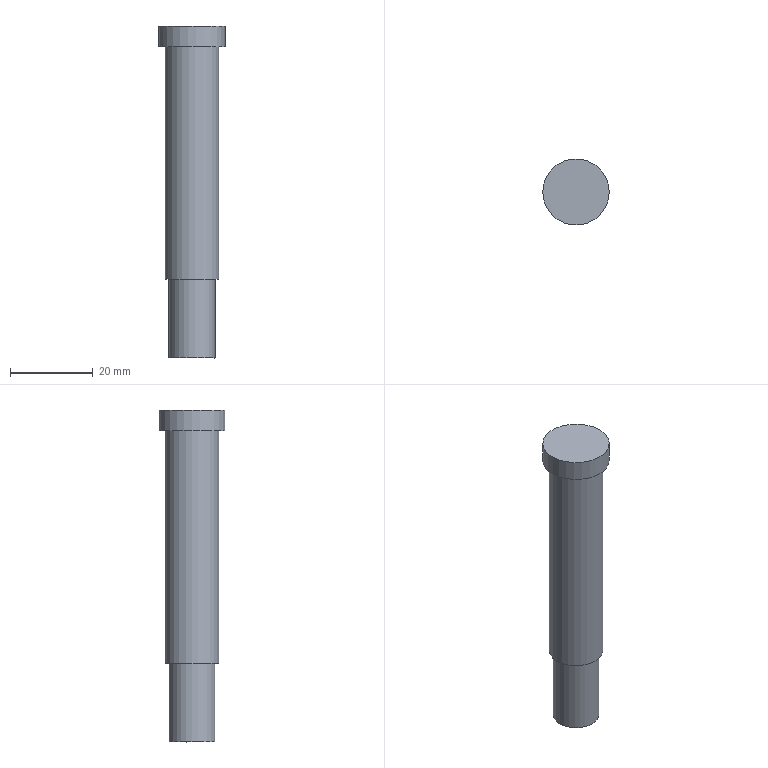Part | NX | features solid 2 | 1 solid | 7 faces | box 16 x 16 x 80 mm | volume 10277 mm3 | plane 4 | cylinder 3 | commonest cylinder face diameters 11.1 x1 13 x1 16 x1
STEP:
#1=CARTESIAN_POINT('',(449.301,141.271,63.192));
#2=VERTEX_POINT('',#1);
#3=CARTESIAN_POINT('',(457.301,141.271,63.192));
#4=DIRECTION('',(-0.000000502,-0.000000149,-1.));
#5=DIRECTION('',(-1.,0.000001668,0.000000502));
#6=AXIS2_PLACEMENT_3D('',#3,#4,#5);
#7=CIRCLE('',#6,8.);
#8=EDGE_CURVE('',#2,#2,#7,.T.);
#9=ORIENTED_EDGE('',*,*,#8,.F.);
#10=EDGE_LOOP('',(#9));
#11=FACE_BOUND('',#10,.T.);
#12=CARTESIAN_POINT('',(457.301,141.271,63.192));
#13=DIRECTION('',(0.000000502,0.000000149,1.));
#14=DIRECTION('',(-1.,0.000001668,0.000000502));
#15=AXIS2_PLACEMENT_3D('',#12,#13,#14);
#16=PLANE('',#15);
#17=ADVANCED_FACE('',(#11),#16,.T.);
#18=CARTESIAN_POINT('',(450.801,141.271,2.192));
#19=VERTEX_POINT('',#18);
#20=CARTESIAN_POINT('',(457.301,141.271,2.192));
#21=DIRECTION('',(-0.000000502,-0.000000149,-1.));
#22=DIRECTION('',(-1.,0.000001668,0.000000502));
#23=AXIS2_PLACEMENT_3D('',#20,#21,#22);
#24=CIRCLE('',#23,6.5);
#25=EDGE_CURVE('',#19,#19,#24,.T.);
#26=ORIENTED_EDGE('',*,*,#25,.F.);
#27=EDGE_LOOP('',(#26));
#28=FACE_BOUND('',#27,.T.);
#29=CARTESIAN_POINT('',(450.801,141.271,58.192));
#30=VERTEX_POINT('',#29);
#31=CARTESIAN_POINT('',(457.301,141.271,58.192));
#32=DIRECTION('',(-0.000000502,-0.000000149,-1.));
#33=DIRECTION('',(-1.,0.000001668,0.000000502));
#34=AXIS2_PLACEMENT_3D('',#31,#32,#33);
#35=CIRCLE('',#34,6.5);
#36=EDGE_CURVE('',#30,#30,#35,.T.);
#37=ORIENTED_EDGE('',*,*,#36,.T.);
#38=EDGE_LOOP('',(#37));
#39=FACE_BOUND('',#38,.T.);
#40=CARTESIAN_POINT('',(457.301,141.271,63.192));
#41=DIRECTION('',(-0.000000502,-0.000000149,-1.));
#42=DIRECTION('',(1.,-0.000001668,-0.000000502));
#43=AXIS2_PLACEMENT_3D('',#40,#41,#42);
#44=CYLINDRICAL_SURFACE('',#43,6.5);
#45=ADVANCED_FACE('',(#28,#39),#44,.T.);
#46=CARTESIAN_POINT('',(451.751,141.271,2.192));
#47=VERTEX_POINT('',#46);
#48=CARTESIAN_POINT('',(457.301,141.271,2.192));
#49=DIRECTION('',(-0.000000502,-0.000000149,-1.));
#50=DIRECTION('',(-1.,0.000001668,0.000000502));
#51=AXIS2_PLACEMENT_3D('',#48,#49,#50);
#52=CIRCLE('',#51,5.55);
#53=EDGE_CURVE('',#47,#47,#52,.T.);
#54=ORIENTED_EDGE('',*,*,#53,.F.);
#55=EDGE_LOOP('',(#54));
#56=FACE_BOUND('',#55,.T.);
#57=ORIENTED_EDGE('',*,*,#25,.T.);
#58=EDGE_LOOP('',(#57));
#59=FACE_BOUND('',#58,.T.);
#60=CARTESIAN_POINT('',(457.301,141.271,2.192));
#61=DIRECTION('',(0.000000502,0.000000149,1.));
#62=DIRECTION('',(-1.,0.000001668,0.000000502));
#63=AXIS2_PLACEMENT_3D('',#60,#61,#62);
#64=PLANE('',#63);
#65=ADVANCED_FACE('',(#56,#59),#64,.F.);
#66=CARTESIAN_POINT('',(449.301,141.271,58.192));
#67=VERTEX_POINT('',#66);
#68=CARTESIAN_POINT('',(457.301,141.271,58.192));
#69=DIRECTION('',(-0.000000502,-0.000000149,-1.));
#70=DIRECTION('',(-1.,0.000001668,0.000000502));
#71=AXIS2_PLACEMENT_3D('',#68,#69,#70);
#72=CIRCLE('',#71,8.);
#73=EDGE_CURVE('',#67,#67,#72,.T.);
#74=ORIENTED_EDGE('',*,*,#73,.T.);
#75=EDGE_LOOP('',(#74));
#76=FACE_BOUND('',#75,.T.);
#77=ORIENTED_EDGE('',*,*,#36,.F.);
#78=EDGE_LOOP('',(#77));
#79=FACE_BOUND('',#78,.T.);
#80=CARTESIAN_POINT('',(457.301,141.271,58.192));
#81=DIRECTION('',(0.000000502,0.000000149,1.));
#82=DIRECTION('',(-1.,0.000001668,0.000000502));
#83=AXIS2_PLACEMENT_3D('',#80,#81,#82);
#84=PLANE('',#83);
#85=ADVANCED_FACE('',(#76,#79),#84,.F.);
#86=ORIENTED_EDGE('',*,*,#73,.F.);
#87=EDGE_LOOP('',(#86));
#88=FACE_BOUND('',#87,.T.);
#89=ORIENTED_EDGE('',*,*,#8,.T.);
#90=EDGE_LOOP('',(#89));
#91=FACE_BOUND('',#90,.T.);
#92=CARTESIAN_POINT('',(457.301,141.271,58.192));
#93=DIRECTION('',(0.000000502,0.000000149,1.));
#94=DIRECTION('',(-1.,0.000001668,0.000000502));
#95=AXIS2_PLACEMENT_3D('',#92,#93,#94);
#96=CYLINDRICAL_SURFACE('',#95,8.);
#97=ADVANCED_FACE('',(#88,#91),#96,.T.);
#98=CARTESIAN_POINT('',(451.751,141.271,-16.808));
#99=VERTEX_POINT('',#98);
#100=CARTESIAN_POINT('',(457.301,141.271,-16.808));
#101=DIRECTION('',(-0.000000502,-0.000000149,-1.));
#102=DIRECTION('',(-1.,0.000001668,0.000000502));
#103=AXIS2_PLACEMENT_3D('',#100,#101,#102);
#104=CIRCLE('',#103,5.55);
#105=EDGE_CURVE('',#99,#99,#104,.T.);
#106=ORIENTED_EDGE('',*,*,#105,.F.);
#107=EDGE_LOOP('',(#106));
#108=FACE_BOUND('',#107,.T.);
#109=ORIENTED_EDGE('',*,*,#53,.T.);
#110=EDGE_LOOP('',(#109));
#111=FACE_BOUND('',#110,.T.);
#112=CARTESIAN_POINT('',(457.301,141.271,-16.808));
#113=DIRECTION('',(0.000000502,0.000000149,1.));
#114=DIRECTION('',(-1.,0.000001668,0.000000502));
#115=AXIS2_PLACEMENT_3D('',#112,#113,#114);
#116=CYLINDRICAL_SURFACE('',#115,5.55);
#117=ADVANCED_FACE('',(#108,#111),#116,.T.);
#118=ORIENTED_EDGE('',*,*,#105,.T.);
#119=EDGE_LOOP('',(#118));
#120=FACE_BOUND('',#119,.T.);
#121=CARTESIAN_POINT('',(457.301,141.271,-16.808));
#122=DIRECTION('',(0.000000502,0.000000149,1.));
#123=DIRECTION('',(-1.,0.000001668,0.000000502));
#124=AXIS2_PLACEMENT_3D('',#121,#122,#123);
#125=PLANE('',#124);
#126=ADVANCED_FACE('',(#120),#125,.F.);
#127=CLOSED_SHELL('',(#17,#45,#65,#85,#97,#117,#126));
#128=MANIFOLD_SOLID_BREP('',#127);
#129=(LENGTH_UNIT()NAMED_UNIT(*)SI_UNIT(.MILLI.,.METRE.));
#130=UNCERTAINTY_MEASURE_WITH_UNIT(LENGTH_MEASURE(0.00001),#129,'','');
#131=(NAMED_UNIT(*)PLANE_ANGLE_UNIT()SI_UNIT($,.RADIAN.));
#132=(NAMED_UNIT(*)SI_UNIT($,.STERADIAN.)SOLID_ANGLE_UNIT());
#133=(GEOMETRIC_REPRESENTATION_CONTEXT(3)GLOBAL_UNCERTAINTY_ASSIGNED_CONTEXT((#130))GLOBAL_UNIT_ASSIGNED_CONTEXT((#129,#131,#132))REPRESENTATION_CONTEXT('',''));
#134=ADVANCED_BREP_SHAPE_REPRESENTATION('',(#128),#133);